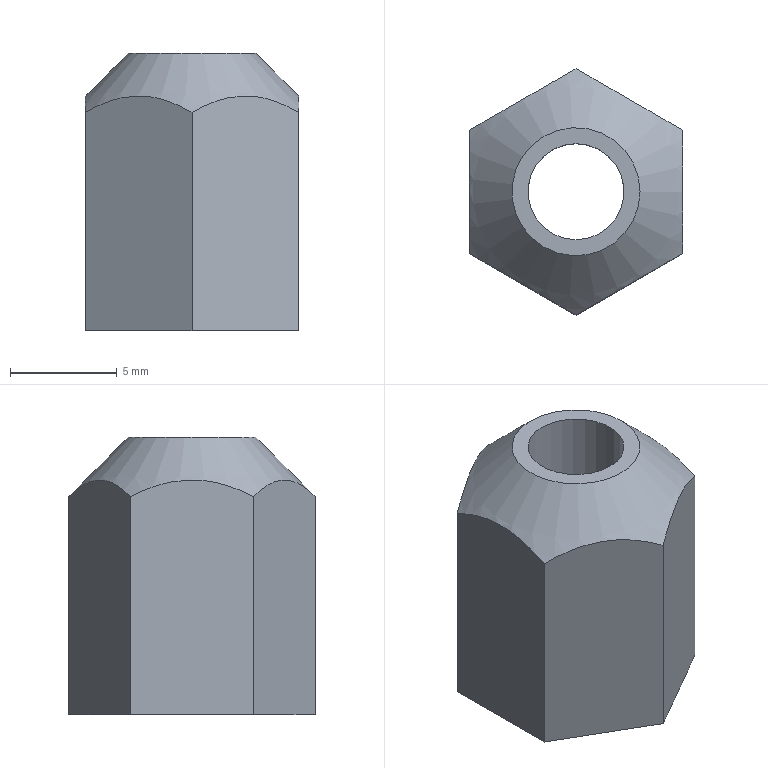Part | STEP file | 1-12.4 | 1 solid | 12 faces | box 10 x 11.547 x 13 mm | volume 537.367 mm3 | plane 9 | cylinder 2 | cone 1 | commonest cylinder face diameters 4.5 x1 8 x1
STEP:
#1=CARTESIAN_POINT('',(0.,0.,0.));
#2=DIRECTION('',(0.,0.,1.));
#3=DIRECTION('',(1.,0.,0.));
#4=AXIS2_PLACEMENT_3D('',#1,#2,#3);
#5=CARTESIAN_POINT('',(0.,5.774,0.));
#6=VERTEX_POINT('',#5);
#7=CARTESIAN_POINT('',(-5.,2.887,0.));
#8=VERTEX_POINT('',#7);
#9=CARTESIAN_POINT('',(0.,5.774,0.));
#10=DIRECTION('',(-0.866,-0.5,0.));
#11=VECTOR('',#10,1.);
#12=LINE('',#9,#11);
#13=CARTESIAN_POINT('',(-2.5,4.33,6.5));
#14=DIRECTION('',(-0.5,0.866,0.));
#15=DIRECTION('',(-0.866,-0.5,0.));
#16=AXIS2_PLACEMENT_3D('',#13,#14,#15);
#17=PLANE('',#16);
#18=CARTESIAN_POINT('',(-2.887,-6.5));
#19=DIRECTION('',(1.,0.));
#20=VECTOR('',#19,1.);
#21=LINE('',#18,#20);
#22=(GEOMETRIC_REPRESENTATION_CONTEXT(2)PARAMETRIC_REPRESENTATION_CONTEXT()REPRESENTATION_CONTEXT('',''));
#23=DEFINITIONAL_REPRESENTATION('',(#21),#22);
#24=PCURVE('',#17,#23);
#25=CARTESIAN_POINT('',(-0.7735,0.,0.));
#26=DIRECTION('',(0.,0.,1.));
#27=DIRECTION('',(0.,1.,0.));
#28=AXIS2_PLACEMENT_3D('',#25,#26,#27);
#29=PLANE('',#28);
#30=CARTESIAN_POINT('',(5.774,-0.7735));
#31=DIRECTION('',(-0.5,0.866));
#32=VECTOR('',#31,1.);
#33=LINE('',#30,#32);
#34=(GEOMETRIC_REPRESENTATION_CONTEXT(2)PARAMETRIC_REPRESENTATION_CONTEXT()REPRESENTATION_CONTEXT('',''));
#35=DEFINITIONAL_REPRESENTATION('',(#33),#34);
#36=PCURVE('',#29,#35);
#37=SURFACE_CURVE('',#12,(#24,#36),.PCURVE_S1.);
#38=EDGE_CURVE('',#6,#8,#37,.T.);
#39=ORIENTED_EDGE('',*,*,#38,.T.);
#40=CARTESIAN_POINT('',(-5.,2.887,10.226));
#41=VERTEX_POINT('',#40);
#42=CARTESIAN_POINT('',(-5.,2.887,0.));
#43=DIRECTION('',(0.,0.,1.));
#44=VECTOR('',#43,1.);
#45=LINE('',#42,#44);
#46=CARTESIAN_POINT('',(2.887,-6.5));
#47=DIRECTION('',(0.,1.));
#48=VECTOR('',#47,1.);
#49=LINE('',#46,#48);
#50=(GEOMETRIC_REPRESENTATION_CONTEXT(2)PARAMETRIC_REPRESENTATION_CONTEXT()REPRESENTATION_CONTEXT('',''));
#51=DEFINITIONAL_REPRESENTATION('',(#49),#50);
#52=PCURVE('',#17,#51);
#53=CARTESIAN_POINT('',(-5.,0.,6.5));
#54=DIRECTION('',(-1.,0.,0.));
#55=DIRECTION('',(0.,-1.,0.));
#56=AXIS2_PLACEMENT_3D('',#53,#54,#55);
#57=PLANE('',#56);
#58=CARTESIAN_POINT('',(-2.887,-6.5));
#59=DIRECTION('',(0.,1.));
#60=VECTOR('',#59,1.);
#61=LINE('',#58,#60);
#62=(GEOMETRIC_REPRESENTATION_CONTEXT(2)PARAMETRIC_REPRESENTATION_CONTEXT()REPRESENTATION_CONTEXT('',''));
#63=DEFINITIONAL_REPRESENTATION('',(#61),#62);
#64=PCURVE('',#57,#63);
#65=SURFACE_CURVE('',#45,(#52,#64),.PCURVE_S1.);
#66=EDGE_CURVE('',#8,#41,#65,.T.);
#67=ORIENTED_EDGE('',*,*,#66,.T.);
#68=CARTESIAN_POINT('',(0.,5.774,10.226));
#69=VERTEX_POINT('',#68);
#70=CARTESIAN_POINT('',(0.,5.774,10.226));
#71=CARTESIAN_POINT('',(-2.5,4.33,11.67));
#72=CARTESIAN_POINT('',(-5.,2.887,10.226));
#73=(BOUNDED_CURVE()B_SPLINE_CURVE(2,(#70,#71,#72),.UNSPECIFIED.,.F.,.F.)B_SPLINE_CURVE_WITH_KNOTS((3,3),(0.,1.),.PIECEWISE_BEZIER_KNOTS.)CURVE()GEOMETRIC_REPRESENTATION_ITEM()RATIONAL_B_SPLINE_CURVE((1.033,1.192,1.033))REPRESENTATION_ITEM(''));
#74=CARTESIAN_POINT('',(-2.887,3.726));
#75=CARTESIAN_POINT('',(0.,5.17));
#76=CARTESIAN_POINT('',(2.887,3.726));
#77=(BOUNDED_CURVE()B_SPLINE_CURVE(2,(#74,#75,#76),.UNSPECIFIED.,.F.,.F.)B_SPLINE_CURVE_WITH_KNOTS((3,3),(0.,1.),.PIECEWISE_BEZIER_KNOTS.)CURVE()GEOMETRIC_REPRESENTATION_ITEM()RATIONAL_B_SPLINE_CURVE((1.033,1.192,1.033))REPRESENTATION_ITEM(''));
#78=(GEOMETRIC_REPRESENTATION_CONTEXT(2)PARAMETRIC_REPRESENTATION_CONTEXT()REPRESENTATION_CONTEXT('',''));
#79=DEFINITIONAL_REPRESENTATION('',(#77),#78);
#80=PCURVE('',#17,#79);
#81=CARTESIAN_POINT('',(0.,0.,13.));
#82=DIRECTION('',(0.,0.,-1.));
#83=DIRECTION('',(1.,0.,0.));
#84=AXIS2_PLACEMENT_3D('',#81,#82,#83);
#85=CONICAL_SURFACE('',#84,3.,0.7854);
#86=CARTESIAN_POINT('',(4.712,2.774));
#87=CARTESIAN_POINT('',(4.697,2.723));
#88=CARTESIAN_POINT('',(4.667,2.628));
#89=CARTESIAN_POINT('',(4.621,2.502));
#90=CARTESIAN_POINT('',(4.574,2.392));
#91=CARTESIAN_POINT('',(4.527,2.297));
#92=CARTESIAN_POINT('',(4.479,2.216));
#93=CARTESIAN_POINT('',(4.431,2.148));
#94=CARTESIAN_POINT('',(4.383,2.094));
#95=CARTESIAN_POINT('',(4.335,2.052));
#96=CARTESIAN_POINT('',(4.286,2.022));
#97=CARTESIAN_POINT('',(4.238,2.004));
#98=CARTESIAN_POINT('',(4.189,1.998));
#99=CARTESIAN_POINT('',(4.14,2.004));
#100=CARTESIAN_POINT('',(4.091,2.022));
#101=CARTESIAN_POINT('',(4.043,2.052));
#102=CARTESIAN_POINT('',(3.994,2.094));
#103=CARTESIAN_POINT('',(3.946,2.148));
#104=CARTESIAN_POINT('',(3.898,2.216));
#105=CARTESIAN_POINT('',(3.851,2.297));
#106=CARTESIAN_POINT('',(3.804,2.392));
#107=CARTESIAN_POINT('',(3.757,2.502));
#108=CARTESIAN_POINT('',(3.711,2.628));
#109=CARTESIAN_POINT('',(3.68,2.723));
#110=CARTESIAN_POINT('',(3.665,2.774));
#111=B_SPLINE_CURVE_WITH_KNOTS('',3,(#86,#87,#88,#89,#90,#91,#92,#93,#94,#95,#96,#97,#98,#99,#100,#101,#102,#103,#104,#105,#106,#107,#108,#109,#110),.UNSPECIFIED.,.F.,.F.,(4,1,1,1,1,1,1,1,1,1,1,1,1,1,1,1,1,1,1,1,1,1,4),(0.,0.04545,0.09091,0.1364,0.1818,0.2273,0.2727,0.3182,0.3636,0.4091,0.4545,0.5,0.5455,0.5909,0.6364,0.6818,0.7273,0.7727,0.8182,0.8636,0.9091,0.9545,1.),.QUASI_UNIFORM_KNOTS.);
#112=(GEOMETRIC_REPRESENTATION_CONTEXT(2)PARAMETRIC_REPRESENTATION_CONTEXT()REPRESENTATION_CONTEXT('',''));
#113=DEFINITIONAL_REPRESENTATION('',(#111),#112);
#114=PCURVE('',#85,#113);
#115=SURFACE_CURVE('',#73,(#80,#114),.PCURVE_S1.);
#116=EDGE_CURVE('',#69,#41,#115,.T.);
#117=ORIENTED_EDGE('',*,*,#116,.F.);
#118=CARTESIAN_POINT('',(0.,5.774,0.));
#119=DIRECTION('',(0.,0.,1.));
#120=VECTOR('',#119,1.);
#121=LINE('',#118,#120);
#122=CARTESIAN_POINT('',(-2.887,-6.5));
#123=DIRECTION('',(0.,1.));
#124=VECTOR('',#123,1.);
#125=LINE('',#122,#124);
#126=(GEOMETRIC_REPRESENTATION_CONTEXT(2)PARAMETRIC_REPRESENTATION_CONTEXT()REPRESENTATION_CONTEXT('',''));
#127=DEFINITIONAL_REPRESENTATION('',(#125),#126);
#128=PCURVE('',#17,#127);
#129=CARTESIAN_POINT('',(2.5,4.33,6.5));
#130=DIRECTION('',(0.5,0.866,0.));
#131=DIRECTION('',(-0.866,0.5,0.));
#132=AXIS2_PLACEMENT_3D('',#129,#130,#131);
#133=PLANE('',#132);
#134=CARTESIAN_POINT('',(2.887,-6.5));
#135=DIRECTION('',(0.,1.));
#136=VECTOR('',#135,1.);
#137=LINE('',#134,#136);
#138=(GEOMETRIC_REPRESENTATION_CONTEXT(2)PARAMETRIC_REPRESENTATION_CONTEXT()REPRESENTATION_CONTEXT('',''));
#139=DEFINITIONAL_REPRESENTATION('',(#137),#138);
#140=PCURVE('',#133,#139);
#141=SURFACE_CURVE('',#121,(#128,#140),.PCURVE_S1.);
#142=EDGE_CURVE('',#6,#69,#141,.T.);
#143=ORIENTED_EDGE('',*,*,#142,.F.);
#144=EDGE_LOOP('',(#39,#67,#117,#143));
#145=FACE_BOUND('',#144,.T.);
#146=ADVANCED_FACE('',(#145),#17,.T.);
#147=CARTESIAN_POINT('',(-5.,-2.887,0.));
#148=VERTEX_POINT('',#147);
#149=CARTESIAN_POINT('',(-5.,2.887,0.));
#150=DIRECTION('',(0.,-1.,0.));
#151=VECTOR('',#150,1.);
#152=LINE('',#149,#151);
#153=CARTESIAN_POINT('',(-2.887,-6.5));
#154=DIRECTION('',(1.,0.));
#155=VECTOR('',#154,1.);
#156=LINE('',#153,#155);
#157=(GEOMETRIC_REPRESENTATION_CONTEXT(2)PARAMETRIC_REPRESENTATION_CONTEXT()REPRESENTATION_CONTEXT('',''));
#158=DEFINITIONAL_REPRESENTATION('',(#156),#157);
#159=PCURVE('',#57,#158);
#160=CARTESIAN_POINT('',(2.887,4.226));
#161=DIRECTION('',(-1.,0.));
#162=VECTOR('',#161,1.);
#163=LINE('',#160,#162);
#164=(GEOMETRIC_REPRESENTATION_CONTEXT(2)PARAMETRIC_REPRESENTATION_CONTEXT()REPRESENTATION_CONTEXT('',''));
#165=DEFINITIONAL_REPRESENTATION('',(#163),#164);
#166=PCURVE('',#29,#165);
#167=SURFACE_CURVE('',#152,(#159,#166),.PCURVE_S1.);
#168=EDGE_CURVE('',#8,#148,#167,.T.);
#169=ORIENTED_EDGE('',*,*,#168,.T.);
#170=CARTESIAN_POINT('',(-5.,-2.887,10.226));
#171=VERTEX_POINT('',#170);
#172=CARTESIAN_POINT('',(-5.,-2.887,0.));
#173=DIRECTION('',(0.,0.,1.));
#174=VECTOR('',#173,1.);
#175=LINE('',#172,#174);
#176=CARTESIAN_POINT('',(2.887,-6.5));
#177=DIRECTION('',(0.,1.));
#178=VECTOR('',#177,1.);
#179=LINE('',#176,#178);
#180=(GEOMETRIC_REPRESENTATION_CONTEXT(2)PARAMETRIC_REPRESENTATION_CONTEXT()REPRESENTATION_CONTEXT('',''));
#181=DEFINITIONAL_REPRESENTATION('',(#179),#180);
#182=PCURVE('',#57,#181);
#183=CARTESIAN_POINT('',(-2.5,-4.33,6.5));
#184=DIRECTION('',(-0.5,-0.866,0.));
#185=DIRECTION('',(0.866,-0.5,0.));
#186=AXIS2_PLACEMENT_3D('',#183,#184,#185);
#187=PLANE('',#186);
#188=CARTESIAN_POINT('',(-2.887,-6.5));
#189=DIRECTION('',(0.,1.));
#190=VECTOR('',#189,1.);
#191=LINE('',#188,#190);
#192=(GEOMETRIC_REPRESENTATION_CONTEXT(2)PARAMETRIC_REPRESENTATION_CONTEXT()REPRESENTATION_CONTEXT('',''));
#193=DEFINITIONAL_REPRESENTATION('',(#191),#192);
#194=PCURVE('',#187,#193);
#195=SURFACE_CURVE('',#175,(#182,#194),.PCURVE_S1.);
#196=EDGE_CURVE('',#148,#171,#195,.T.);
#197=ORIENTED_EDGE('',*,*,#196,.T.);
#198=CARTESIAN_POINT('',(-5.,2.887,10.226));
#199=CARTESIAN_POINT('',(-5.,0.,11.67));
#200=CARTESIAN_POINT('',(-5.,-2.887,10.226));
#201=(BOUNDED_CURVE()B_SPLINE_CURVE(2,(#198,#199,#200),.UNSPECIFIED.,.F.,.F.)B_SPLINE_CURVE_WITH_KNOTS((3,3),(0.,1.),.PIECEWISE_BEZIER_KNOTS.)CURVE()GEOMETRIC_REPRESENTATION_ITEM()RATIONAL_B_SPLINE_CURVE((1.033,1.192,1.033))REPRESENTATION_ITEM(''));
#202=CARTESIAN_POINT('',(-2.887,3.726));
#203=CARTESIAN_POINT('',(0.,5.17));
#204=CARTESIAN_POINT('',(2.887,3.726));
#205=(BOUNDED_CURVE()B_SPLINE_CURVE(2,(#202,#203,#204),.UNSPECIFIED.,.F.,.F.)B_SPLINE_CURVE_WITH_KNOTS((3,3),(0.,1.),.PIECEWISE_BEZIER_KNOTS.)CURVE()GEOMETRIC_REPRESENTATION_ITEM()RATIONAL_B_SPLINE_CURVE((1.033,1.192,1.033))REPRESENTATION_ITEM(''));
#206=(GEOMETRIC_REPRESENTATION_CONTEXT(2)PARAMETRIC_REPRESENTATION_CONTEXT()REPRESENTATION_CONTEXT('',''));
#207=DEFINITIONAL_REPRESENTATION('',(#205),#206);
#208=PCURVE('',#57,#207);
#209=CARTESIAN_POINT('',(3.665,2.774));
#210=CARTESIAN_POINT('',(3.65,2.723));
#211=CARTESIAN_POINT('',(3.62,2.628));
#212=CARTESIAN_POINT('',(3.573,2.502));
#213=CARTESIAN_POINT('',(3.527,2.392));
#214=CARTESIAN_POINT('',(3.479,2.297));
#215=CARTESIAN_POINT('',(3.432,2.216));
#216=CARTESIAN_POINT('',(3.384,2.148));
#217=CARTESIAN_POINT('',(3.336,2.094));
#218=CARTESIAN_POINT('',(3.288,2.052));
#219=CARTESIAN_POINT('',(3.239,2.022));
#220=CARTESIAN_POINT('',(3.19,2.004));
#221=CARTESIAN_POINT('',(3.142,1.998));
#222=CARTESIAN_POINT('',(3.093,2.004));
#223=CARTESIAN_POINT('',(3.044,2.022));
#224=CARTESIAN_POINT('',(2.996,2.052));
#225=CARTESIAN_POINT('',(2.947,2.094));
#226=CARTESIAN_POINT('',(2.899,2.148));
#227=CARTESIAN_POINT('',(2.851,2.216));
#228=CARTESIAN_POINT('',(2.804,2.297));
#229=CARTESIAN_POINT('',(2.757,2.392));
#230=CARTESIAN_POINT('',(2.71,2.502));
#231=CARTESIAN_POINT('',(2.664,2.628));
#232=CARTESIAN_POINT('',(2.633,2.723));
#233=CARTESIAN_POINT('',(2.618,2.774));
#234=B_SPLINE_CURVE_WITH_KNOTS('',3,(#209,#210,#211,#212,#213,#214,#215,#216,#217,#218,#219,#220,#221,#222,#223,#224,#225,#226,#227,#228,#229,#230,#231,#232,#233),.UNSPECIFIED.,.F.,.F.,(4,1,1,1,1,1,1,1,1,1,1,1,1,1,1,1,1,1,1,1,1,1,4),(0.,0.04545,0.09091,0.1364,0.1818,0.2273,0.2727,0.3182,0.3636,0.4091,0.4545,0.5,0.5455,0.5909,0.6364,0.6818,0.7273,0.7727,0.8182,0.8636,0.9091,0.9545,1.),.QUASI_UNIFORM_KNOTS.);
#235=(GEOMETRIC_REPRESENTATION_CONTEXT(2)PARAMETRIC_REPRESENTATION_CONTEXT()REPRESENTATION_CONTEXT('',''));
#236=DEFINITIONAL_REPRESENTATION('',(#234),#235);
#237=PCURVE('',#85,#236);
#238=SURFACE_CURVE('',#201,(#208,#237),.PCURVE_S1.);
#239=EDGE_CURVE('',#41,#171,#238,.T.);
#240=ORIENTED_EDGE('',*,*,#239,.F.);
#241=ORIENTED_EDGE('',*,*,#66,.F.);
#242=EDGE_LOOP('',(#169,#197,#240,#241));
#243=FACE_BOUND('',#242,.T.);
#244=ADVANCED_FACE('',(#243),#57,.T.);
#245=CARTESIAN_POINT('',(0.,-5.774,0.));
#246=VERTEX_POINT('',#245);
#247=CARTESIAN_POINT('',(-5.,-2.887,0.));
#248=DIRECTION('',(0.866,-0.5,0.));
#249=VECTOR('',#248,1.);
#250=LINE('',#247,#249);
#251=CARTESIAN_POINT('',(-2.887,-6.5));
#252=DIRECTION('',(1.,0.));
#253=VECTOR('',#252,1.);
#254=LINE('',#251,#253);
#255=(GEOMETRIC_REPRESENTATION_CONTEXT(2)PARAMETRIC_REPRESENTATION_CONTEXT()REPRESENTATION_CONTEXT('',''));
#256=DEFINITIONAL_REPRESENTATION('',(#254),#255);
#257=PCURVE('',#187,#256);
#258=CARTESIAN_POINT('',(-2.887,4.226));
#259=DIRECTION('',(-0.5,-0.866));
#260=VECTOR('',#259,1.);
#261=LINE('',#258,#260);
#262=(GEOMETRIC_REPRESENTATION_CONTEXT(2)PARAMETRIC_REPRESENTATION_CONTEXT()REPRESENTATION_CONTEXT('',''));
#263=DEFINITIONAL_REPRESENTATION('',(#261),#262);
#264=PCURVE('',#29,#263);
#265=SURFACE_CURVE('',#250,(#257,#264),.PCURVE_S1.);
#266=EDGE_CURVE('',#148,#246,#265,.T.);
#267=ORIENTED_EDGE('',*,*,#266,.T.);
#268=CARTESIAN_POINT('',(0.,-5.774,10.226));
#269=VERTEX_POINT('',#268);
#270=CARTESIAN_POINT('',(0.,-5.774,0.));
#271=DIRECTION('',(0.,0.,1.));
#272=VECTOR('',#271,1.);
#273=LINE('',#270,#272);
#274=CARTESIAN_POINT('',(2.887,-6.5));
#275=DIRECTION('',(0.,1.));
#276=VECTOR('',#275,1.);
#277=LINE('',#274,#276);
#278=(GEOMETRIC_REPRESENTATION_CONTEXT(2)PARAMETRIC_REPRESENTATION_CONTEXT()REPRESENTATION_CONTEXT('',''));
#279=DEFINITIONAL_REPRESENTATION('',(#277),#278);
#280=PCURVE('',#187,#279);
#281=CARTESIAN_POINT('',(2.5,-4.33,6.5));
#282=DIRECTION('',(0.5,-0.866,0.));
#283=DIRECTION('',(0.866,0.5,0.));
#284=AXIS2_PLACEMENT_3D('',#281,#282,#283);
#285=PLANE('',#284);
#286=CARTESIAN_POINT('',(-2.887,-6.5));
#287=DIRECTION('',(0.,1.));
#288=VECTOR('',#287,1.);
#289=LINE('',#286,#288);
#290=(GEOMETRIC_REPRESENTATION_CONTEXT(2)PARAMETRIC_REPRESENTATION_CONTEXT()REPRESENTATION_CONTEXT('',''));
#291=DEFINITIONAL_REPRESENTATION('',(#289),#290);
#292=PCURVE('',#285,#291);
#293=SURFACE_CURVE('',#273,(#280,#292),.PCURVE_S1.);
#294=EDGE_CURVE('',#246,#269,#293,.T.);
#295=ORIENTED_EDGE('',*,*,#294,.T.);
#296=CARTESIAN_POINT('',(-5.,-2.887,10.226));
#297=CARTESIAN_POINT('',(-2.5,-4.33,11.67));
#298=CARTESIAN_POINT('',(0.,-5.774,10.226));
#299=(BOUNDED_CURVE()B_SPLINE_CURVE(2,(#296,#297,#298),.UNSPECIFIED.,.F.,.F.)B_SPLINE_CURVE_WITH_KNOTS((3,3),(0.,1.),.PIECEWISE_BEZIER_KNOTS.)CURVE()GEOMETRIC_REPRESENTATION_ITEM()RATIONAL_B_SPLINE_CURVE((1.033,1.192,1.033))REPRESENTATION_ITEM(''));
#300=CARTESIAN_POINT('',(-2.887,3.726));
#301=CARTESIAN_POINT('',(0.,5.17));
#302=CARTESIAN_POINT('',(2.887,3.726));
#303=(BOUNDED_CURVE()B_SPLINE_CURVE(2,(#300,#301,#302),.UNSPECIFIED.,.F.,.F.)B_SPLINE_CURVE_WITH_KNOTS((3,3),(0.,1.),.PIECEWISE_BEZIER_KNOTS.)CURVE()GEOMETRIC_REPRESENTATION_ITEM()RATIONAL_B_SPLINE_CURVE((1.033,1.192,1.033))REPRESENTATION_ITEM(''));
#304=(GEOMETRIC_REPRESENTATION_CONTEXT(2)PARAMETRIC_REPRESENTATION_CONTEXT()REPRESENTATION_CONTEXT('',''));
#305=DEFINITIONAL_REPRESENTATION('',(#303),#304);
#306=PCURVE('',#187,#305);
#307=CARTESIAN_POINT('',(2.618,2.774));
#308=CARTESIAN_POINT('',(2.603,2.723));
#309=CARTESIAN_POINT('',(2.572,2.628));
#310=CARTESIAN_POINT('',(2.526,2.502));
#311=CARTESIAN_POINT('',(2.479,2.392));
#312=CARTESIAN_POINT('',(2.432,2.297));
#313=CARTESIAN_POINT('',(2.385,2.216));
#314=CARTESIAN_POINT('',(2.337,2.148));
#315=CARTESIAN_POINT('',(2.289,2.094));
#316=CARTESIAN_POINT('',(2.24,2.052));
#317=CARTESIAN_POINT('',(2.192,2.022));
#318=CARTESIAN_POINT('',(2.143,2.004));
#319=CARTESIAN_POINT('',(2.094,1.998));
#320=CARTESIAN_POINT('',(2.046,2.004));
#321=CARTESIAN_POINT('',(1.997,2.022));
#322=CARTESIAN_POINT('',(1.948,2.052));
#323=CARTESIAN_POINT('',(1.9,2.094));
#324=CARTESIAN_POINT('',(1.852,2.148));
#325=CARTESIAN_POINT('',(1.804,2.216));
#326=CARTESIAN_POINT('',(1.757,2.297));
#327=CARTESIAN_POINT('',(1.709,2.392));
#328=CARTESIAN_POINT('',(1.663,2.502));
#329=CARTESIAN_POINT('',(1.616,2.628));
#330=CARTESIAN_POINT('',(1.586,2.723));
#331=CARTESIAN_POINT('',(1.571,2.774));
#332=B_SPLINE_CURVE_WITH_KNOTS('',3,(#307,#308,#309,#310,#311,#312,#313,#314,#315,#316,#317,#318,#319,#320,#321,#322,#323,#324,#325,#326,#327,#328,#329,#330,#331),.UNSPECIFIED.,.F.,.F.,(4,1,1,1,1,1,1,1,1,1,1,1,1,1,1,1,1,1,1,1,1,1,4),(0.,0.04545,0.09091,0.1364,0.1818,0.2273,0.2727,0.3182,0.3636,0.4091,0.4545,0.5,0.5455,0.5909,0.6364,0.6818,0.7273,0.7727,0.8182,0.8636,0.9091,0.9545,1.),.QUASI_UNIFORM_KNOTS.);
#333=(GEOMETRIC_REPRESENTATION_CONTEXT(2)PARAMETRIC_REPRESENTATION_CONTEXT()REPRESENTATION_CONTEXT('',''));
#334=DEFINITIONAL_REPRESENTATION('',(#332),#333);
#335=PCURVE('',#85,#334);
#336=SURFACE_CURVE('',#299,(#306,#335),.PCURVE_S1.);
#337=EDGE_CURVE('',#171,#269,#336,.T.);
#338=ORIENTED_EDGE('',*,*,#337,.F.);
#339=ORIENTED_EDGE('',*,*,#196,.F.);
#340=EDGE_LOOP('',(#267,#295,#338,#339));
#341=FACE_BOUND('',#340,.T.);
#342=ADVANCED_FACE('',(#341),#187,.T.);
#343=CARTESIAN_POINT('',(5.,-2.887,0.));
#344=VERTEX_POINT('',#343);
#345=CARTESIAN_POINT('',(0.,-5.774,0.));
#346=DIRECTION('',(0.866,0.5,0.));
#347=VECTOR('',#346,1.);
#348=LINE('',#345,#347);
#349=CARTESIAN_POINT('',(-2.887,-6.5));
#350=DIRECTION('',(1.,0.));
#351=VECTOR('',#350,1.);
#352=LINE('',#349,#351);
#353=(GEOMETRIC_REPRESENTATION_CONTEXT(2)PARAMETRIC_REPRESENTATION_CONTEXT()REPRESENTATION_CONTEXT('',''));
#354=DEFINITIONAL_REPRESENTATION('',(#352),#353);
#355=PCURVE('',#285,#354);
#356=CARTESIAN_POINT('',(-5.774,-0.7735));
#357=DIRECTION('',(0.5,-0.866));
#358=VECTOR('',#357,1.);
#359=LINE('',#356,#358);
#360=(GEOMETRIC_REPRESENTATION_CONTEXT(2)PARAMETRIC_REPRESENTATION_CONTEXT()REPRESENTATION_CONTEXT('',''));
#361=DEFINITIONAL_REPRESENTATION('',(#359),#360);
#362=PCURVE('',#29,#361);
#363=SURFACE_CURVE('',#348,(#355,#362),.PCURVE_S1.);
#364=EDGE_CURVE('',#246,#344,#363,.T.);
#365=ORIENTED_EDGE('',*,*,#364,.T.);
#366=CARTESIAN_POINT('',(5.,-2.887,10.226));
#367=VERTEX_POINT('',#366);
#368=CARTESIAN_POINT('',(5.,-2.887,0.));
#369=DIRECTION('',(0.,0.,1.));
#370=VECTOR('',#369,1.);
#371=LINE('',#368,#370);
#372=CARTESIAN_POINT('',(2.887,-6.5));
#373=DIRECTION('',(0.,1.));
#374=VECTOR('',#373,1.);
#375=LINE('',#372,#374);
#376=(GEOMETRIC_REPRESENTATION_CONTEXT(2)PARAMETRIC_REPRESENTATION_CONTEXT()REPRESENTATION_CONTEXT('',''));
#377=DEFINITIONAL_REPRESENTATION('',(#375),#376);
#378=PCURVE('',#285,#377);
#379=CARTESIAN_POINT('',(5.,0.,6.5));
#380=DIRECTION('',(1.,0.,0.));
#381=DIRECTION('',(0.,1.,0.));
#382=AXIS2_PLACEMENT_3D('',#379,#380,#381);
#383=PLANE('',#382);
#384=CARTESIAN_POINT('',(-2.887,-6.5));
#385=DIRECTION('',(0.,1.));
#386=VECTOR('',#385,1.);
#387=LINE('',#384,#386);
#388=(GEOMETRIC_REPRESENTATION_CONTEXT(2)PARAMETRIC_REPRESENTATION_CONTEXT()REPRESENTATION_CONTEXT('',''));
#389=DEFINITIONAL_REPRESENTATION('',(#387),#388);
#390=PCURVE('',#383,#389);
#391=SURFACE_CURVE('',#371,(#378,#390),.PCURVE_S1.);
#392=EDGE_CURVE('',#344,#367,#391,.T.);
#393=ORIENTED_EDGE('',*,*,#392,.T.);
#394=CARTESIAN_POINT('',(0.,-5.774,10.226));
#395=CARTESIAN_POINT('',(2.5,-4.33,11.67));
#396=CARTESIAN_POINT('',(5.,-2.887,10.226));
#397=(BOUNDED_CURVE()B_SPLINE_CURVE(2,(#394,#395,#396),.UNSPECIFIED.,.F.,.F.)B_SPLINE_CURVE_WITH_KNOTS((3,3),(0.,1.),.PIECEWISE_BEZIER_KNOTS.)CURVE()GEOMETRIC_REPRESENTATION_ITEM()RATIONAL_B_SPLINE_CURVE((1.033,1.192,1.033))REPRESENTATION_ITEM(''));
#398=CARTESIAN_POINT('',(-2.887,3.726));
#399=CARTESIAN_POINT('',(0.,5.17));
#400=CARTESIAN_POINT('',(2.887,3.726));
#401=(BOUNDED_CURVE()B_SPLINE_CURVE(2,(#398,#399,#400),.UNSPECIFIED.,.F.,.F.)B_SPLINE_CURVE_WITH_KNOTS((3,3),(0.,1.),.PIECEWISE_BEZIER_KNOTS.)CURVE()GEOMETRIC_REPRESENTATION_ITEM()RATIONAL_B_SPLINE_CURVE((1.033,1.192,1.033))REPRESENTATION_ITEM(''));
#402=(GEOMETRIC_REPRESENTATION_CONTEXT(2)PARAMETRIC_REPRESENTATION_CONTEXT()REPRESENTATION_CONTEXT('',''));
#403=DEFINITIONAL_REPRESENTATION('',(#401),#402);
#404=PCURVE('',#285,#403);
#405=CARTESIAN_POINT('',(1.571,2.774));
#406=CARTESIAN_POINT('',(1.556,2.723));
#407=CARTESIAN_POINT('',(1.525,2.628));
#408=CARTESIAN_POINT('',(1.479,2.502));
#409=CARTESIAN_POINT('',(1.432,2.392));
#410=CARTESIAN_POINT('',(1.385,2.297));
#411=CARTESIAN_POINT('',(1.338,2.216));
#412=CARTESIAN_POINT('',(1.29,2.148));
#413=CARTESIAN_POINT('',(1.241,2.094));
#414=CARTESIAN_POINT('',(1.193,2.052));
#415=CARTESIAN_POINT('',(1.145,2.022));
#416=CARTESIAN_POINT('',(1.096,2.004));
#417=CARTESIAN_POINT('',(1.047,1.998));
#418=CARTESIAN_POINT('',(0.9985,2.004));
#419=CARTESIAN_POINT('',(0.9498,2.022));
#420=CARTESIAN_POINT('',(0.9013,2.052));
#421=CARTESIAN_POINT('',(0.8529,2.094));
#422=CARTESIAN_POINT('',(0.8048,2.148));
#423=CARTESIAN_POINT('',(0.7569,2.216));
#424=CARTESIAN_POINT('',(0.7094,2.297));
#425=CARTESIAN_POINT('',(0.6622,2.392));
#426=CARTESIAN_POINT('',(0.6155,2.502));
#427=CARTESIAN_POINT('',(0.5692,2.628));
#428=CARTESIAN_POINT('',(0.5388,2.723));
#429=CARTESIAN_POINT('',(0.5236,2.774));
#430=B_SPLINE_CURVE_WITH_KNOTS('',3,(#405,#406,#407,#408,#409,#410,#411,#412,#413,#414,#415,#416,#417,#418,#419,#420,#421,#422,#423,#424,#425,#426,#427,#428,#429),.UNSPECIFIED.,.F.,.F.,(4,1,1,1,1,1,1,1,1,1,1,1,1,1,1,1,1,1,1,1,1,1,4),(0.,0.04545,0.09091,0.1364,0.1818,0.2273,0.2727,0.3182,0.3636,0.4091,0.4545,0.5,0.5455,0.5909,0.6364,0.6818,0.7273,0.7727,0.8182,0.8636,0.9091,0.9545,1.),.QUASI_UNIFORM_KNOTS.);
#431=(GEOMETRIC_REPRESENTATION_CONTEXT(2)PARAMETRIC_REPRESENTATION_CONTEXT()REPRESENTATION_CONTEXT('',''));
#432=DEFINITIONAL_REPRESENTATION('',(#430),#431);
#433=PCURVE('',#85,#432);
#434=SURFACE_CURVE('',#397,(#404,#433),.PCURVE_S1.);
#435=EDGE_CURVE('',#269,#367,#434,.T.);
#436=ORIENTED_EDGE('',*,*,#435,.F.);
#437=ORIENTED_EDGE('',*,*,#294,.F.);
#438=EDGE_LOOP('',(#365,#393,#436,#437));
#439=FACE_BOUND('',#438,.T.);
#440=ADVANCED_FACE('',(#439),#285,.T.);
#441=CARTESIAN_POINT('',(5.,2.887,0.));
#442=VERTEX_POINT('',#441);
#443=CARTESIAN_POINT('',(5.,-2.887,0.));
#444=DIRECTION('',(0.,1.,0.));
#445=VECTOR('',#444,1.);
#446=LINE('',#443,#445);
#447=CARTESIAN_POINT('',(-2.887,-6.5));
#448=DIRECTION('',(1.,0.));
#449=VECTOR('',#448,1.);
#450=LINE('',#447,#449);
#451=(GEOMETRIC_REPRESENTATION_CONTEXT(2)PARAMETRIC_REPRESENTATION_CONTEXT()REPRESENTATION_CONTEXT('',''));
#452=DEFINITIONAL_REPRESENTATION('',(#450),#451);
#453=PCURVE('',#383,#452);
#454=CARTESIAN_POINT('',(-2.887,-5.774));
#455=DIRECTION('',(1.,0.));
#456=VECTOR('',#455,1.);
#457=LINE('',#454,#456);
#458=(GEOMETRIC_REPRESENTATION_CONTEXT(2)PARAMETRIC_REPRESENTATION_CONTEXT()REPRESENTATION_CONTEXT('',''));
#459=DEFINITIONAL_REPRESENTATION('',(#457),#458);
#460=PCURVE('',#29,#459);
#461=SURFACE_CURVE('',#446,(#453,#460),.PCURVE_S1.);
#462=EDGE_CURVE('',#344,#442,#461,.T.);
#463=ORIENTED_EDGE('',*,*,#462,.T.);
#464=CARTESIAN_POINT('',(5.,2.887,10.226));
#465=VERTEX_POINT('',#464);
#466=CARTESIAN_POINT('',(5.,2.887,0.));
#467=DIRECTION('',(0.,0.,1.));
#468=VECTOR('',#467,1.);
#469=LINE('',#466,#468);
#470=CARTESIAN_POINT('',(2.887,-6.5));
#471=DIRECTION('',(0.,1.));
#472=VECTOR('',#471,1.);
#473=LINE('',#470,#472);
#474=(GEOMETRIC_REPRESENTATION_CONTEXT(2)PARAMETRIC_REPRESENTATION_CONTEXT()REPRESENTATION_CONTEXT('',''));
#475=DEFINITIONAL_REPRESENTATION('',(#473),#474);
#476=PCURVE('',#383,#475);
#477=CARTESIAN_POINT('',(-2.887,-6.5));
#478=DIRECTION('',(0.,1.));
#479=VECTOR('',#478,1.);
#480=LINE('',#477,#479);
#481=(GEOMETRIC_REPRESENTATION_CONTEXT(2)PARAMETRIC_REPRESENTATION_CONTEXT()REPRESENTATION_CONTEXT('',''));
#482=DEFINITIONAL_REPRESENTATION('',(#480),#481);
#483=PCURVE('',#133,#482);
#484=SURFACE_CURVE('',#469,(#476,#483),.PCURVE_S1.);
#485=EDGE_CURVE('',#442,#465,#484,.T.);
#486=ORIENTED_EDGE('',*,*,#485,.T.);
#487=CARTESIAN_POINT('',(5.,0.,11.));
#488=VERTEX_POINT('',#487);
#489=CARTESIAN_POINT('',(5.,0.,11.));
#490=CARTESIAN_POINT('',(5.,1.34,11.));
#491=CARTESIAN_POINT('',(5.,2.887,10.226));
#492=(BOUNDED_CURVE()B_SPLINE_CURVE(2,(#489,#490,#491),.UNSPECIFIED.,.F.,.F.)B_SPLINE_CURVE_WITH_KNOTS((3,3),(0.,1.),.PIECEWISE_BEZIER_KNOTS.)CURVE()GEOMETRIC_REPRESENTATION_ITEM()RATIONAL_B_SPLINE_CURVE((1.113,1.113,1.033))REPRESENTATION_ITEM(''));
#493=CARTESIAN_POINT('',(0.,4.5));
#494=CARTESIAN_POINT('',(1.34,4.5));
#495=CARTESIAN_POINT('',(2.887,3.726));
#496=(BOUNDED_CURVE()B_SPLINE_CURVE(2,(#493,#494,#495),.UNSPECIFIED.,.F.,.F.)B_SPLINE_CURVE_WITH_KNOTS((3,3),(0.,1.),.PIECEWISE_BEZIER_KNOTS.)CURVE()GEOMETRIC_REPRESENTATION_ITEM()RATIONAL_B_SPLINE_CURVE((1.113,1.113,1.033))REPRESENTATION_ITEM(''));
#497=(GEOMETRIC_REPRESENTATION_CONTEXT(2)PARAMETRIC_REPRESENTATION_CONTEXT()REPRESENTATION_CONTEXT('',''));
#498=DEFINITIONAL_REPRESENTATION('',(#496),#497);
#499=PCURVE('',#383,#498);
#500=CARTESIAN_POINT('',(6.283,2.));
#501=CARTESIAN_POINT('',(6.275,2.));
#502=CARTESIAN_POINT('',(6.259,2.001));
#503=CARTESIAN_POINT('',(6.234,2.005));
#504=CARTESIAN_POINT('',(6.21,2.013));
#505=CARTESIAN_POINT('',(6.186,2.023));
#506=CARTESIAN_POINT('',(6.162,2.037));
#507=CARTESIAN_POINT('',(6.137,2.053));
#508=CARTESIAN_POINT('',(6.113,2.073));
#509=CARTESIAN_POINT('',(6.089,2.095));
#510=CARTESIAN_POINT('',(6.065,2.121));
#511=CARTESIAN_POINT('',(6.041,2.15));
#512=CARTESIAN_POINT('',(6.017,2.182));
#513=CARTESIAN_POINT('',(5.993,2.218));
#514=CARTESIAN_POINT('',(5.969,2.257));
#515=CARTESIAN_POINT('',(5.945,2.299));
#516=CARTESIAN_POINT('',(5.922,2.345));
#517=CARTESIAN_POINT('',(5.898,2.394));
#518=CARTESIAN_POINT('',(5.875,2.447));
#519=CARTESIAN_POINT('',(5.852,2.504));
#520=CARTESIAN_POINT('',(5.828,2.565));
#521=CARTESIAN_POINT('',(5.805,2.63));
#522=CARTESIAN_POINT('',(5.782,2.699));
#523=CARTESIAN_POINT('',(5.767,2.748));
#524=CARTESIAN_POINT('',(5.76,2.774));
#525=B_SPLINE_CURVE_WITH_KNOTS('',3,(#500,#501,#502,#503,#504,#505,#506,#507,#508,#509,#510,#511,#512,#513,#514,#515,#516,#517,#518,#519,#520,#521,#522,#523,#524),.UNSPECIFIED.,.F.,.F.,(4,1,1,1,1,1,1,1,1,1,1,1,1,1,1,1,1,1,1,1,1,1,4),(0.,0.04545,0.09091,0.1364,0.1818,0.2273,0.2727,0.3182,0.3636,0.4091,0.4545,0.5,0.5455,0.5909,0.6364,0.6818,0.7273,0.7727,0.8182,0.8636,0.9091,0.9545,1.),.QUASI_UNIFORM_KNOTS.);
#526=(GEOMETRIC_REPRESENTATION_CONTEXT(2)PARAMETRIC_REPRESENTATION_CONTEXT()REPRESENTATION_CONTEXT('',''));
#527=DEFINITIONAL_REPRESENTATION('',(#525),#526);
#528=PCURVE('',#85,#527);
#529=SURFACE_CURVE('',#492,(#499,#528),.PCURVE_S1.);
#530=EDGE_CURVE('',#488,#465,#529,.T.);
#531=ORIENTED_EDGE('',*,*,#530,.F.);
#532=CARTESIAN_POINT('',(5.,-2.887,10.226));
#533=CARTESIAN_POINT('',(5.,-1.34,11.));
#534=CARTESIAN_POINT('',(5.,0.,11.));
#535=(BOUNDED_CURVE()B_SPLINE_CURVE(2,(#532,#533,#534),.UNSPECIFIED.,.F.,.F.)B_SPLINE_CURVE_WITH_KNOTS((3,3),(0.,1.),.PIECEWISE_BEZIER_KNOTS.)CURVE()GEOMETRIC_REPRESENTATION_ITEM()RATIONAL_B_SPLINE_CURVE((1.033,1.113,1.113))REPRESENTATION_ITEM(''));
#536=CARTESIAN_POINT('',(-2.887,3.726));
#537=CARTESIAN_POINT('',(-1.34,4.5));
#538=CARTESIAN_POINT('',(0.,4.5));
#539=(BOUNDED_CURVE()B_SPLINE_CURVE(2,(#536,#537,#538),.UNSPECIFIED.,.F.,.F.)B_SPLINE_CURVE_WITH_KNOTS((3,3),(0.,1.),.PIECEWISE_BEZIER_KNOTS.)CURVE()GEOMETRIC_REPRESENTATION_ITEM()RATIONAL_B_SPLINE_CURVE((1.033,1.113,1.113))REPRESENTATION_ITEM(''));
#540=(GEOMETRIC_REPRESENTATION_CONTEXT(2)PARAMETRIC_REPRESENTATION_CONTEXT()REPRESENTATION_CONTEXT('',''));
#541=DEFINITIONAL_REPRESENTATION('',(#539),#540);
#542=PCURVE('',#383,#541);
#543=CARTESIAN_POINT('',(0.5236,2.774));
#544=CARTESIAN_POINT('',(0.516,2.748));
#545=CARTESIAN_POINT('',(0.5008,2.699));
#546=CARTESIAN_POINT('',(0.4779,2.63));
#547=CARTESIAN_POINT('',(0.4548,2.565));
#548=CARTESIAN_POINT('',(0.4317,2.504));
#549=CARTESIAN_POINT('',(0.4084,2.447));
#550=CARTESIAN_POINT('',(0.3849,2.394));
#551=CARTESIAN_POINT('',(0.3614,2.345));
#552=CARTESIAN_POINT('',(0.3378,2.299));
#553=CARTESIAN_POINT('',(0.3141,2.257));
#554=CARTESIAN_POINT('',(0.2903,2.218));
#555=CARTESIAN_POINT('',(0.2664,2.182));
#556=CARTESIAN_POINT('',(0.2424,2.15));
#557=CARTESIAN_POINT('',(0.2184,2.121));
#558=CARTESIAN_POINT('',(0.1943,2.095));
#559=CARTESIAN_POINT('',(0.1701,2.073));
#560=CARTESIAN_POINT('',(0.1459,2.053));
#561=CARTESIAN_POINT('',(0.1217,2.037));
#562=CARTESIAN_POINT('',(0.09736,2.023));
#563=CARTESIAN_POINT('',(0.07305,2.013));
#564=CARTESIAN_POINT('',(0.04871,2.005));
#565=CARTESIAN_POINT('',(0.02436,2.001));
#566=CARTESIAN_POINT('',(0.00812,2.));
#567=CARTESIAN_POINT('',(0.,2.));
#568=B_SPLINE_CURVE_WITH_KNOTS('',3,(#543,#544,#545,#546,#547,#548,#549,#550,#551,#552,#553,#554,#555,#556,#557,#558,#559,#560,#561,#562,#563,#564,#565,#566,#567),.UNSPECIFIED.,.F.,.F.,(4,1,1,1,1,1,1,1,1,1,1,1,1,1,1,1,1,1,1,1,1,1,4),(0.,0.04545,0.09091,0.1364,0.1818,0.2273,0.2727,0.3182,0.3636,0.4091,0.4545,0.5,0.5455,0.5909,0.6364,0.6818,0.7273,0.7727,0.8182,0.8636,0.9091,0.9545,1.),.QUASI_UNIFORM_KNOTS.);
#569=(GEOMETRIC_REPRESENTATION_CONTEXT(2)PARAMETRIC_REPRESENTATION_CONTEXT()REPRESENTATION_CONTEXT('',''));
#570=DEFINITIONAL_REPRESENTATION('',(#568),#569);
#571=PCURVE('',#85,#570);
#572=SURFACE_CURVE('',#535,(#542,#571),.PCURVE_S1.);
#573=EDGE_CURVE('',#367,#488,#572,.T.);
#574=ORIENTED_EDGE('',*,*,#573,.F.);
#575=ORIENTED_EDGE('',*,*,#392,.F.);
#576=EDGE_LOOP('',(#463,#486,#531,#574,#575));
#577=FACE_BOUND('',#576,.T.);
#578=ADVANCED_FACE('',(#577),#383,.T.);
#579=CARTESIAN_POINT('',(5.,2.887,0.));
#580=DIRECTION('',(-0.866,0.5,0.));
#581=VECTOR('',#580,1.);
#582=LINE('',#579,#581);
#583=CARTESIAN_POINT('',(-2.887,-6.5));
#584=DIRECTION('',(1.,0.));
#585=VECTOR('',#584,1.);
#586=LINE('',#583,#585);
#587=(GEOMETRIC_REPRESENTATION_CONTEXT(2)PARAMETRIC_REPRESENTATION_CONTEXT()REPRESENTATION_CONTEXT('',''));
#588=DEFINITIONAL_REPRESENTATION('',(#586),#587);
#589=PCURVE('',#133,#588);
#590=CARTESIAN_POINT('',(2.887,-5.774));
#591=DIRECTION('',(0.5,0.866));
#592=VECTOR('',#591,1.);
#593=LINE('',#590,#592);
#594=(GEOMETRIC_REPRESENTATION_CONTEXT(2)PARAMETRIC_REPRESENTATION_CONTEXT()REPRESENTATION_CONTEXT('',''));
#595=DEFINITIONAL_REPRESENTATION('',(#593),#594);
#596=PCURVE('',#29,#595);
#597=SURFACE_CURVE('',#582,(#589,#596),.PCURVE_S1.);
#598=EDGE_CURVE('',#442,#6,#597,.T.);
#599=ORIENTED_EDGE('',*,*,#598,.T.);
#600=ORIENTED_EDGE('',*,*,#142,.T.);
#601=CARTESIAN_POINT('',(5.,2.887,10.226));
#602=CARTESIAN_POINT('',(2.5,4.33,11.67));
#603=CARTESIAN_POINT('',(0.,5.774,10.226));
#604=(BOUNDED_CURVE()B_SPLINE_CURVE(2,(#601,#602,#603),.UNSPECIFIED.,.F.,.F.)B_SPLINE_CURVE_WITH_KNOTS((3,3),(0.,1.),.PIECEWISE_BEZIER_KNOTS.)CURVE()GEOMETRIC_REPRESENTATION_ITEM()RATIONAL_B_SPLINE_CURVE((1.033,1.192,1.033))REPRESENTATION_ITEM(''));
#605=CARTESIAN_POINT('',(-2.887,3.726));
#606=CARTESIAN_POINT('',(0.,5.17));
#607=CARTESIAN_POINT('',(2.887,3.726));
#608=(BOUNDED_CURVE()B_SPLINE_CURVE(2,(#605,#606,#607),.UNSPECIFIED.,.F.,.F.)B_SPLINE_CURVE_WITH_KNOTS((3,3),(0.,1.),.PIECEWISE_BEZIER_KNOTS.)CURVE()GEOMETRIC_REPRESENTATION_ITEM()RATIONAL_B_SPLINE_CURVE((1.033,1.192,1.033))REPRESENTATION_ITEM(''));
#609=(GEOMETRIC_REPRESENTATION_CONTEXT(2)PARAMETRIC_REPRESENTATION_CONTEXT()REPRESENTATION_CONTEXT('',''));
#610=DEFINITIONAL_REPRESENTATION('',(#608),#609);
#611=PCURVE('',#133,#610);
#612=CARTESIAN_POINT('',(5.76,2.774));
#613=CARTESIAN_POINT('',(5.744,2.723));
#614=CARTESIAN_POINT('',(5.714,2.628));
#615=CARTESIAN_POINT('',(5.668,2.502));
#616=CARTESIAN_POINT('',(5.621,2.392));
#617=CARTESIAN_POINT('',(5.574,2.297));
#618=CARTESIAN_POINT('',(5.526,2.216));
#619=CARTESIAN_POINT('',(5.478,2.148));
#620=CARTESIAN_POINT('',(5.43,2.094));
#621=CARTESIAN_POINT('',(5.382,2.052));
#622=CARTESIAN_POINT('',(5.333,2.022));
#623=CARTESIAN_POINT('',(5.285,2.004));
#624=CARTESIAN_POINT('',(5.236,1.998));
#625=CARTESIAN_POINT('',(5.187,2.004));
#626=CARTESIAN_POINT('',(5.139,2.022));
#627=CARTESIAN_POINT('',(5.09,2.052));
#628=CARTESIAN_POINT('',(5.042,2.094));
#629=CARTESIAN_POINT('',(4.994,2.148));
#630=CARTESIAN_POINT('',(4.946,2.216));
#631=CARTESIAN_POINT('',(4.898,2.297));
#632=CARTESIAN_POINT('',(4.851,2.392));
#633=CARTESIAN_POINT('',(4.804,2.502));
#634=CARTESIAN_POINT('',(4.758,2.628));
#635=CARTESIAN_POINT('',(4.728,2.723));
#636=CARTESIAN_POINT('',(4.712,2.774));
#637=B_SPLINE_CURVE_WITH_KNOTS('',3,(#612,#613,#614,#615,#616,#617,#618,#619,#620,#621,#622,#623,#624,#625,#626,#627,#628,#629,#630,#631,#632,#633,#634,#635,#636),.UNSPECIFIED.,.F.,.F.,(4,1,1,1,1,1,1,1,1,1,1,1,1,1,1,1,1,1,1,1,1,1,4),(0.,0.04545,0.09091,0.1364,0.1818,0.2273,0.2727,0.3182,0.3636,0.4091,0.4545,0.5,0.5455,0.5909,0.6364,0.6818,0.7273,0.7727,0.8182,0.8636,0.9091,0.9545,1.),.QUASI_UNIFORM_KNOTS.);
#638=(GEOMETRIC_REPRESENTATION_CONTEXT(2)PARAMETRIC_REPRESENTATION_CONTEXT()REPRESENTATION_CONTEXT('',''));
#639=DEFINITIONAL_REPRESENTATION('',(#637),#638);
#640=PCURVE('',#85,#639);
#641=SURFACE_CURVE('',#604,(#611,#640),.PCURVE_S1.);
#642=EDGE_CURVE('',#465,#69,#641,.T.);
#643=ORIENTED_EDGE('',*,*,#642,.F.);
#644=ORIENTED_EDGE('',*,*,#485,.F.);
#645=EDGE_LOOP('',(#599,#600,#643,#644));
#646=FACE_BOUND('',#645,.T.);
#647=ADVANCED_FACE('',(#646),#133,.T.);
#648=CARTESIAN_POINT('',(3.,0.,13.));
#649=VERTEX_POINT('',#648);
#650=CARTESIAN_POINT('',(3.,0.,13.));
#651=DIRECTION('',(0.7071,0.,-0.7071));
#652=VECTOR('',#651,1.);
#653=LINE('',#650,#652);
#654=CARTESIAN_POINT('',(6.283,0.));
#655=DIRECTION('',(0.,1.));
#656=VECTOR('',#655,1.);
#657=LINE('',#654,#656);
#658=(GEOMETRIC_REPRESENTATION_CONTEXT(2)PARAMETRIC_REPRESENTATION_CONTEXT()REPRESENTATION_CONTEXT('',''));
#659=DEFINITIONAL_REPRESENTATION('',(#657),#658);
#660=PCURVE('',#85,#659);
#661=CARTESIAN_POINT('',(0.,0.));
#662=DIRECTION('',(0.,1.));
#663=VECTOR('',#662,1.);
#664=LINE('',#661,#663);
#665=(GEOMETRIC_REPRESENTATION_CONTEXT(2)PARAMETRIC_REPRESENTATION_CONTEXT()REPRESENTATION_CONTEXT('',''));
#666=DEFINITIONAL_REPRESENTATION('',(#664),#665);
#667=PCURVE('',#85,#666);
#668=SEAM_CURVE('',#653,(#660,#667),.PCURVE_S1.);
#669=EDGE_CURVE('',#649,#488,#668,.T.);
#670=ORIENTED_EDGE('',*,*,#669,.T.);
#671=ORIENTED_EDGE('',*,*,#530,.T.);
#672=ORIENTED_EDGE('',*,*,#642,.T.);
#673=ORIENTED_EDGE('',*,*,#116,.T.);
#674=ORIENTED_EDGE('',*,*,#239,.T.);
#675=ORIENTED_EDGE('',*,*,#337,.T.);
#676=ORIENTED_EDGE('',*,*,#435,.T.);
#677=ORIENTED_EDGE('',*,*,#573,.T.);
#678=ORIENTED_EDGE('',*,*,#669,.F.);
#679=CARTESIAN_POINT('',(0.,0.,13.));
#680=DIRECTION('',(0.,0.,1.));
#681=DIRECTION('',(1.,0.,0.));
#682=AXIS2_PLACEMENT_3D('',#679,#680,#681);
#683=CIRCLE('',#682,3.);
#684=CARTESIAN_POINT('',(6.283,0.));
#685=DIRECTION('',(-1.,0.));
#686=VECTOR('',#685,1.);
#687=LINE('',#684,#686);
#688=(GEOMETRIC_REPRESENTATION_CONTEXT(2)PARAMETRIC_REPRESENTATION_CONTEXT()REPRESENTATION_CONTEXT('',''));
#689=DEFINITIONAL_REPRESENTATION('',(#687),#688);
#690=PCURVE('',#85,#689);
#691=CARTESIAN_POINT('',(-0.7735,0.,13.));
#692=DIRECTION('',(0.,0.,1.));
#693=DIRECTION('',(0.,1.,0.));
#694=AXIS2_PLACEMENT_3D('',#691,#692,#693);
#695=PLANE('',#694);
#696=CARTESIAN_POINT('',(0.,-0.7735));
#697=DIRECTION('',(0.,-1.));
#698=AXIS2_PLACEMENT_2D('',#696,#697);
#699=CIRCLE('',#698,3.);
#700=(GEOMETRIC_REPRESENTATION_CONTEXT(2)PARAMETRIC_REPRESENTATION_CONTEXT()REPRESENTATION_CONTEXT('',''));
#701=DEFINITIONAL_REPRESENTATION('',(#699),#700);
#702=PCURVE('',#695,#701);
#703=SURFACE_CURVE('',#683,(#690,#702),.PCURVE_S1.);
#704=EDGE_CURVE('',#649,#649,#703,.T.);
#705=ORIENTED_EDGE('',*,*,#704,.F.);
#706=EDGE_LOOP('',(#670,#671,#672,#673,#674,#675,#676,#677,#678,#705));
#707=FACE_BOUND('',#706,.T.);
#708=ADVANCED_FACE('',(#707),#85,.T.);
#709=ORIENTED_EDGE('',*,*,#704,.T.);
#710=EDGE_LOOP('',(#709));
#711=FACE_BOUND('',#710,.T.);
#712=CARTESIAN_POINT('',(0.,-2.25,13.));
#713=VERTEX_POINT('',#712);
#714=CARTESIAN_POINT('',(0.,0.,13.));
#715=DIRECTION('',(0.,0.,1.));
#716=DIRECTION('',(0.,-1.,0.));
#717=AXIS2_PLACEMENT_3D('',#714,#715,#716);
#718=CIRCLE('',#717,2.25);
#719=CARTESIAN_POINT('',(0.,-0.7735));
#720=DIRECTION('',(-1.,0.));
#721=AXIS2_PLACEMENT_2D('',#719,#720);
#722=CIRCLE('',#721,2.25);
#723=(GEOMETRIC_REPRESENTATION_CONTEXT(2)PARAMETRIC_REPRESENTATION_CONTEXT()REPRESENTATION_CONTEXT('',''));
#724=DEFINITIONAL_REPRESENTATION('',(#722),#723);
#725=PCURVE('',#695,#724);
#726=CARTESIAN_POINT('',(0.,0.,13.));
#727=DIRECTION('',(0.,0.,-1.));
#728=DIRECTION('',(0.,-1.,0.));
#729=AXIS2_PLACEMENT_3D('',#726,#727,#728);
#730=CYLINDRICAL_SURFACE('',#729,2.25);
#731=CARTESIAN_POINT('',(6.283,0.));
#732=DIRECTION('',(-1.,0.));
#733=VECTOR('',#732,1.);
#734=LINE('',#731,#733);
#735=(GEOMETRIC_REPRESENTATION_CONTEXT(2)PARAMETRIC_REPRESENTATION_CONTEXT()REPRESENTATION_CONTEXT('',''));
#736=DEFINITIONAL_REPRESENTATION('',(#734),#735);
#737=PCURVE('',#730,#736);
#738=SURFACE_CURVE('',#718,(#725,#737),.PCURVE_S1.);
#739=EDGE_CURVE('',#713,#713,#738,.T.);
#740=ORIENTED_EDGE('',*,*,#739,.F.);
#741=EDGE_LOOP('',(#740));
#742=FACE_BOUND('',#741,.T.);
#743=ADVANCED_FACE('',(#711,#742),#695,.T.);
#744=ORIENTED_EDGE('',*,*,#38,.T.);
#745=ORIENTED_EDGE('',*,*,#168,.T.);
#746=ORIENTED_EDGE('',*,*,#266,.T.);
#747=ORIENTED_EDGE('',*,*,#364,.T.);
#748=ORIENTED_EDGE('',*,*,#462,.T.);
#749=ORIENTED_EDGE('',*,*,#598,.T.);
#750=EDGE_LOOP('',(#744,#745,#746,#747,#748,#749));
#751=FACE_BOUND('',#750,.F.);
#752=CARTESIAN_POINT('',(0.,-4.,0.));
#753=VERTEX_POINT('',#752);
#754=CARTESIAN_POINT('',(0.,0.,0.));
#755=DIRECTION('',(0.,0.,-1.));
#756=DIRECTION('',(0.,-1.,0.));
#757=AXIS2_PLACEMENT_3D('',#754,#755,#756);
#758=CIRCLE('',#757,4.);
#759=CARTESIAN_POINT('',(-4.,-0.7735));
#760=CARTESIAN_POINT('',(-4.,6.155));
#761=CARTESIAN_POINT('',(2.,2.691));
#762=CARTESIAN_POINT('',(8.,-0.7735));
#763=CARTESIAN_POINT('',(2.,-4.238));
#764=CARTESIAN_POINT('',(-4.,-7.702));
#765=CARTESIAN_POINT('',(-4.,-0.7735));
#766=(BOUNDED_CURVE()B_SPLINE_CURVE(2,(#759,#760,#761,#762,#763,#764,#765),.UNSPECIFIED.,.T.,.F.)B_SPLINE_CURVE_WITH_KNOTS((1,2,2,2,2,1),(-2.094,0.,2.094,4.189,6.283,8.378),.UNSPECIFIED.)CURVE()GEOMETRIC_REPRESENTATION_ITEM()RATIONAL_B_SPLINE_CURVE((1.,0.5,1.,0.5,1.,0.5,1.))REPRESENTATION_ITEM(''));
#767=(GEOMETRIC_REPRESENTATION_CONTEXT(2)PARAMETRIC_REPRESENTATION_CONTEXT()REPRESENTATION_CONTEXT('',''));
#768=DEFINITIONAL_REPRESENTATION('',(#766),#767);
#769=PCURVE('',#29,#768);
#770=CARTESIAN_POINT('',(0.,0.,0.));
#771=DIRECTION('',(0.,0.,1.));
#772=DIRECTION('',(0.,-1.,0.));
#773=AXIS2_PLACEMENT_3D('',#770,#771,#772);
#774=CYLINDRICAL_SURFACE('',#773,4.);
#775=CARTESIAN_POINT('',(6.283,0.));
#776=DIRECTION('',(-1.,0.));
#777=VECTOR('',#776,1.);
#778=LINE('',#775,#777);
#779=(GEOMETRIC_REPRESENTATION_CONTEXT(2)PARAMETRIC_REPRESENTATION_CONTEXT()REPRESENTATION_CONTEXT('',''));
#780=DEFINITIONAL_REPRESENTATION('',(#778),#779);
#781=PCURVE('',#774,#780);
#782=SURFACE_CURVE('',#758,(#769,#781),.PCURVE_S1.);
#783=EDGE_CURVE('',#753,#753,#782,.T.);
#784=ORIENTED_EDGE('',*,*,#783,.T.);
#785=EDGE_LOOP('',(#784));
#786=FACE_BOUND('',#785,.F.);
#787=ADVANCED_FACE('',(#751,#786),#29,.F.);
#788=CARTESIAN_POINT('',(0.,-2.25,9.));
#789=VERTEX_POINT('',#788);
#790=CARTESIAN_POINT('',(0.,-2.25,13.));
#791=DIRECTION('',(0.,0.,-1.));
#792=VECTOR('',#791,1.);
#793=LINE('',#790,#792);
#794=CARTESIAN_POINT('',(6.283,0.));
#795=DIRECTION('',(0.,1.));
#796=VECTOR('',#795,1.);
#797=LINE('',#794,#796);
#798=(GEOMETRIC_REPRESENTATION_CONTEXT(2)PARAMETRIC_REPRESENTATION_CONTEXT()REPRESENTATION_CONTEXT('',''));
#799=DEFINITIONAL_REPRESENTATION('',(#797),#798);
#800=PCURVE('',#730,#799);
#801=CARTESIAN_POINT('',(0.,0.));
#802=DIRECTION('',(0.,1.));
#803=VECTOR('',#802,1.);
#804=LINE('',#801,#803);
#805=(GEOMETRIC_REPRESENTATION_CONTEXT(2)PARAMETRIC_REPRESENTATION_CONTEXT()REPRESENTATION_CONTEXT('',''));
#806=DEFINITIONAL_REPRESENTATION('',(#804),#805);
#807=PCURVE('',#730,#806);
#808=SEAM_CURVE('',#793,(#800,#807),.PCURVE_S1.);
#809=EDGE_CURVE('',#713,#789,#808,.T.);
#810=ORIENTED_EDGE('',*,*,#809,.T.);
#811=CARTESIAN_POINT('',(0.,0.,9.));
#812=DIRECTION('',(0.,0.,1.));
#813=DIRECTION('',(0.,-1.,0.));
#814=AXIS2_PLACEMENT_3D('',#811,#812,#813);
#815=CIRCLE('',#814,2.25);
#816=CARTESIAN_POINT('',(6.283,4.));
#817=DIRECTION('',(-1.,0.));
#818=VECTOR('',#817,1.);
#819=LINE('',#816,#818);
#820=(GEOMETRIC_REPRESENTATION_CONTEXT(2)PARAMETRIC_REPRESENTATION_CONTEXT()REPRESENTATION_CONTEXT('',''));
#821=DEFINITIONAL_REPRESENTATION('',(#819),#820);
#822=PCURVE('',#730,#821);
#823=CARTESIAN_POINT('',(0.,1.072,9.));
#824=DIRECTION('',(0.,0.,-1.));
#825=DIRECTION('',(0.,-1.,0.));
#826=AXIS2_PLACEMENT_3D('',#823,#824,#825);
#827=PLANE('',#826);
#828=CARTESIAN_POINT('',(3.322,0.));
#829=CARTESIAN_POINT('',(3.322,-3.897));
#830=CARTESIAN_POINT('',(-0.0532,-1.949));
#831=CARTESIAN_POINT('',(-3.428,0.));
#832=CARTESIAN_POINT('',(-0.0532,1.949));
#833=CARTESIAN_POINT('',(3.322,3.897));
#834=CARTESIAN_POINT('',(3.322,0.));
#835=(BOUNDED_CURVE()B_SPLINE_CURVE(2,(#828,#829,#830,#831,#832,#833,#834),.UNSPECIFIED.,.T.,.F.)B_SPLINE_CURVE_WITH_KNOTS((1,2,2,2,2,1),(-2.094,0.,2.094,4.189,6.283,8.378),.UNSPECIFIED.)CURVE()GEOMETRIC_REPRESENTATION_ITEM()RATIONAL_B_SPLINE_CURVE((1.,0.5,1.,0.5,1.,0.5,1.))REPRESENTATION_ITEM(''));
#836=(GEOMETRIC_REPRESENTATION_CONTEXT(2)PARAMETRIC_REPRESENTATION_CONTEXT()REPRESENTATION_CONTEXT('',''));
#837=DEFINITIONAL_REPRESENTATION('',(#835),#836);
#838=PCURVE('',#827,#837);
#839=SURFACE_CURVE('',#815,(#822,#838),.PCURVE_S1.);
#840=EDGE_CURVE('',#789,#789,#839,.T.);
#841=ORIENTED_EDGE('',*,*,#840,.T.);
#842=ORIENTED_EDGE('',*,*,#809,.F.);
#843=ORIENTED_EDGE('',*,*,#739,.F.);
#844=EDGE_LOOP('',(#810,#841,#842,#843));
#845=FACE_BOUND('',#844,.F.);
#846=ADVANCED_FACE('',(#845),#730,.F.);
#847=CARTESIAN_POINT('',(0.,-4.,9.));
#848=VERTEX_POINT('',#847);
#849=CARTESIAN_POINT('',(0.,-4.,0.));
#850=DIRECTION('',(0.,0.,1.));
#851=VECTOR('',#850,1.);
#852=LINE('',#849,#851);
#853=CARTESIAN_POINT('',(6.283,0.));
#854=DIRECTION('',(0.,1.));
#855=VECTOR('',#854,1.);
#856=LINE('',#853,#855);
#857=(GEOMETRIC_REPRESENTATION_CONTEXT(2)PARAMETRIC_REPRESENTATION_CONTEXT()REPRESENTATION_CONTEXT('',''));
#858=DEFINITIONAL_REPRESENTATION('',(#856),#857);
#859=PCURVE('',#774,#858);
#860=CARTESIAN_POINT('',(0.,0.));
#861=DIRECTION('',(0.,1.));
#862=VECTOR('',#861,1.);
#863=LINE('',#860,#862);
#864=(GEOMETRIC_REPRESENTATION_CONTEXT(2)PARAMETRIC_REPRESENTATION_CONTEXT()REPRESENTATION_CONTEXT('',''));
#865=DEFINITIONAL_REPRESENTATION('',(#863),#864);
#866=PCURVE('',#774,#865);
#867=SEAM_CURVE('',#852,(#859,#866),.PCURVE_S1.);
#868=EDGE_CURVE('',#753,#848,#867,.T.);
#869=ORIENTED_EDGE('',*,*,#868,.T.);
#870=CARTESIAN_POINT('',(0.,0.,9.));
#871=DIRECTION('',(0.,0.,-1.));
#872=DIRECTION('',(0.,-1.,0.));
#873=AXIS2_PLACEMENT_3D('',#870,#871,#872);
#874=CIRCLE('',#873,4.);
#875=CARTESIAN_POINT('',(6.283,9.));
#876=DIRECTION('',(-1.,0.));
#877=VECTOR('',#876,1.);
#878=LINE('',#875,#877);
#879=(GEOMETRIC_REPRESENTATION_CONTEXT(2)PARAMETRIC_REPRESENTATION_CONTEXT()REPRESENTATION_CONTEXT('',''));
#880=DEFINITIONAL_REPRESENTATION('',(#878),#879);
#881=PCURVE('',#774,#880);
#882=CARTESIAN_POINT('',(1.072,0.));
#883=DIRECTION('',(1.,0.));
#884=AXIS2_PLACEMENT_2D('',#882,#883);
#885=CIRCLE('',#884,4.);
#886=(GEOMETRIC_REPRESENTATION_CONTEXT(2)PARAMETRIC_REPRESENTATION_CONTEXT()REPRESENTATION_CONTEXT('',''));
#887=DEFINITIONAL_REPRESENTATION('',(#885),#886);
#888=PCURVE('',#827,#887);
#889=SURFACE_CURVE('',#874,(#881,#888),.PCURVE_S1.);
#890=EDGE_CURVE('',#848,#848,#889,.T.);
#891=ORIENTED_EDGE('',*,*,#890,.T.);
#892=ORIENTED_EDGE('',*,*,#868,.F.);
#893=ORIENTED_EDGE('',*,*,#783,.F.);
#894=EDGE_LOOP('',(#869,#891,#892,#893));
#895=FACE_BOUND('',#894,.F.);
#896=ADVANCED_FACE('',(#895),#774,.F.);
#897=ORIENTED_EDGE('',*,*,#890,.T.);
#898=EDGE_LOOP('',(#897));
#899=FACE_BOUND('',#898,.T.);
#900=ORIENTED_EDGE('',*,*,#840,.T.);
#901=EDGE_LOOP('',(#900));
#902=FACE_BOUND('',#901,.T.);
#903=ADVANCED_FACE('',(#899,#902),#827,.T.);
#904=CLOSED_SHELL('',(#146,#244,#342,#440,#578,#647,#708,#743,#787,#846,#896,#903));
#905=MANIFOLD_SOLID_BREP('',#904);
#906=(LENGTH_UNIT()NAMED_UNIT(*)SI_UNIT(.MILLI.,.METRE.));
#907=UNCERTAINTY_MEASURE_WITH_UNIT(LENGTH_MEASURE(0.0000001),#906,'','');
#908=(NAMED_UNIT(*)PLANE_ANGLE_UNIT()SI_UNIT($,.RADIAN.));
#909=(NAMED_UNIT(*)SI_UNIT($,.STERADIAN.)SOLID_ANGLE_UNIT());
#910=(GEOMETRIC_REPRESENTATION_CONTEXT(3)GLOBAL_UNCERTAINTY_ASSIGNED_CONTEXT((#907))GLOBAL_UNIT_ASSIGNED_CONTEXT((#906,#908,#909))REPRESENTATION_CONTEXT('',''));
#911=ADVANCED_BREP_SHAPE_REPRESENTATION('',(#4,#905),#910);